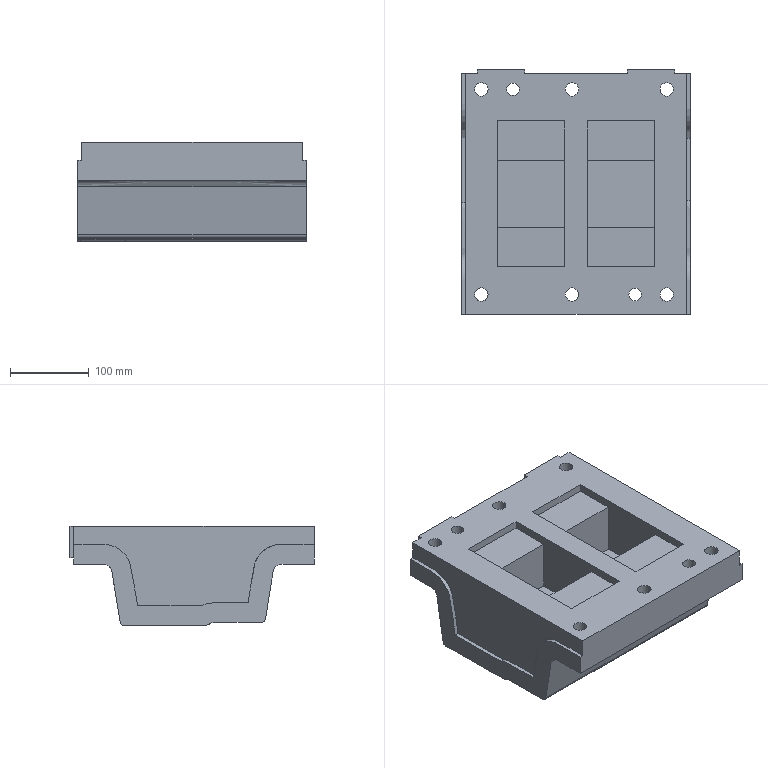Part | NX | features solid 2 | 1 solid | 101 faces | box 290 x 310 x 126.004 mm | volume 7008065 mm3 | plane 46 | spline 31 | cylinder 22 | torus 1 | cone 1 | commonest cylinder face diameters 17 x6 26 x6 10 x3 12 x3 16 x2 14 x1